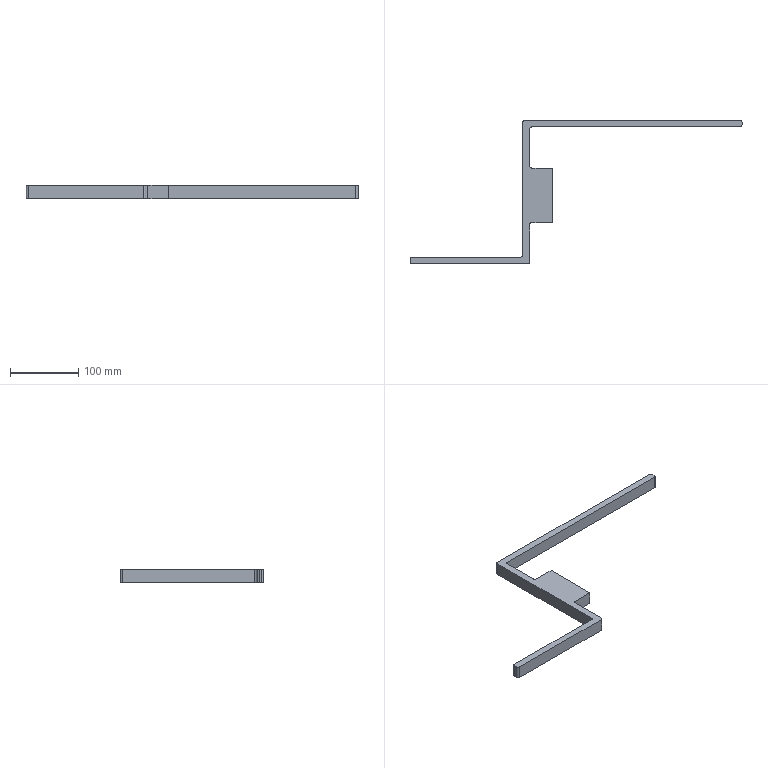Part | STEP file | SN10_015_001_CHAPA_DOBRADA | 1 solid | 30 faces | box 485 x 210 x 19 mm | volume 177968 mm3 | plane 14 | cylinder 13 | cone 3 | commonest cylinder face diameters 6 x10 6.647 x1 8.647 x1 10 x1